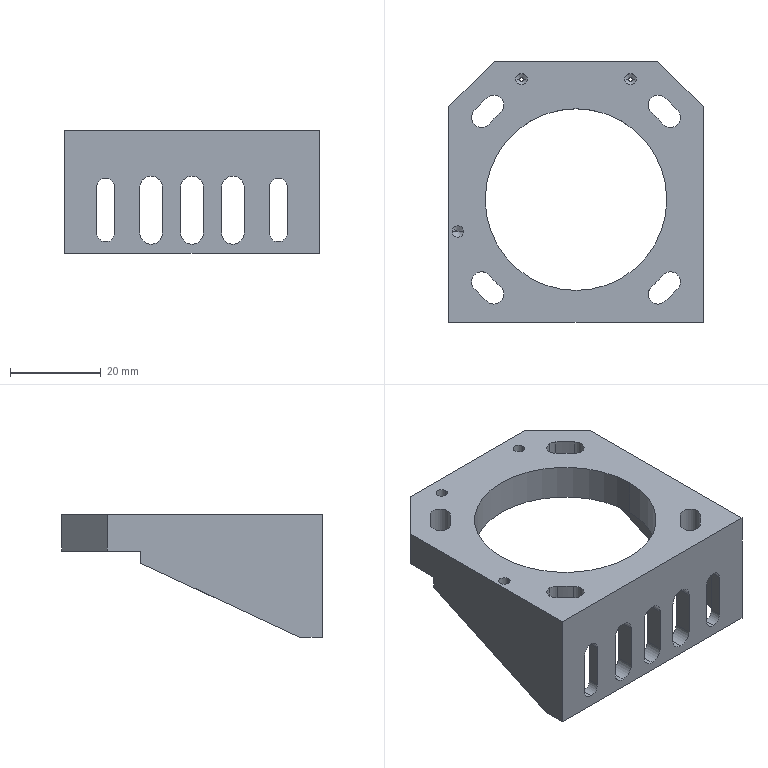NC program | NX | posted with a generic post | part box 56 x 57.4 x 27 mm
Lines 2971 to 3091 of 3091:
(PLANAR_MILL_COPY_COPY_COPY_1 , TOOL : D6A45)
N5934 T07 M6
N5936 G54
N5938 G17 G0 G90 X-1.555 Y-19.935 B0. C0. S7500 M3
N5940 G43 Z30. H7
N5942 Z0.5
N5944 G94 G1 X-1.259 Y-20.1 Z0.409 F1250.
N5946 X4. Z-1.
N5948 X9.
N5950 G3 X10.1 Y-19. R1.1
N5952 X9. Y-17.9 R1.1
N5954 G1 X-1.
N5956 G3 X-2.1 Y-19. R1.1
N5958 X-1. Y-20.1 R1.1
N5960 G1 X4.
N5962 G3 X4.866 Y-19.6 R1.
N5964 G1 Z0.5
N5966 G0 Z30.
N5968 X2.73 Y-9.4
N5970 Z0.5
N5972 G1 Z-1.
N5974 X3.134 Y-10.1
N5976 G3 X4. Y-10.6 R1.
N5978 G1 X9.
N5980 G3 X10.6 Y-9. R1.6
N5982 X9. Y-7.4 R1.6
N5984 G1 X-1.
N5986 G3 X-2.6 Y-9. R1.6
N5988 X-1. Y-10.6 R1.6
N5990 G1 X4.
N5992 G3 X4.866 Y-10.1 R1.
N5994 G1 X5.27 Y-9.4
N5996 Z0.5
N5998 G0 Z30.
N6000 X2.73 Y-0.4
N6002 Z0.5
N6004 G1 Z-1.
N6006 X3.134 Y-1.1
N6008 G3 X4. Y-1.6 R1.
N6010 G1 X9.
N6012 G3 X10.6 Y0. R1.6
N6014 X9. Y1.6 R1.6
N6016 G1 X-1.
N6018 G3 X-2.6 Y0. R1.6
N6020 X-1. Y-1.6 R1.6
N6022 G1 X4.
N6024 G3 X4.866 Y-1.1 R1.
N6026 G1 X5.27 Y-0.4
N6028 Z0.5
N6030 G0 Z30.
N6032 X2.73 Y8.6
N6034 Z0.5
N6036 G1 Z-1.
N6038 X3.134 Y7.9
N6040 G3 X4. Y7.4 R1.
N6042 G1 X9.
N6044 G3 X10.6 Y9. R1.6
N6046 X9. Y10.6 R1.6
N6048 G1 X-1.
N6050 G3 X-2.6 Y9. R1.6
N6052 X-1. Y7.4 R1.6
N6054 G1 X4.
N6056 G3 X4.866 Y7.9 R1.
N6058 G1 X5.27 Y8.6
N6060 Z0.5
N6062 G0 Z30.
N6064 X9.555 Y19.935
N6066 Z0.5
N6068 G1 X9.259 Y20.1 Z0.409
N6070 X4. Z-1.
N6072 X-1.
N6074 G3 X-2.1 Y19. R1.1
N6076 X-1. Y17.9 R1.1
N6078 G1 X9.
N6080 G3 X10.1 Y19. R1.1
N6082 X9. Y20.1 R1.1
N6084 G1 X4.
N6086 G3 X3.134 Y19.6 R1.
N6088 G1 Z0.5
N6090 G0 Z30.
N6092 M5
(刀补 , TOOL : D3)
N6094 T03 M6
N6096 G54
N6098 G17 G0 G90 X9.098 Y19.433 B0. C0. S7500 M3
N6100 G43 Z30. H3
N6102 Z1.
N6104 G94 G1 Z-4. F1000.
N6106 G41 X9. Y19.45 D3
N6108 X-1.
N6110 G3 X-1.45 Y19. R0.45
N6112 X-1. Y18.55 R0.45
N6114 G1 X9.
N6116 G3 X9.45 Y19. R0.45
N6118 X9. Y19.45 R0.45
N6120 X8.74 Y19.3 R0.3
N6122 G40
N6124 G1 X8.706 Y19.206
N6126 Z-3.
N6128 G0 Z30.
N6130 X-1.098 Y-19.433
N6132 Z1.
N6134 G1 Z-4.
N6136 G41 X-1. Y-19.45
N6138 X9.
N6140 G3 X9.45 Y-19. R0.45
N6142 X9. Y-18.55 R0.45
N6144 G1 X-1.
N6146 G3 X-1.45 Y-19. R0.45
N6148 X-1. Y-19.45 R0.45
N6150 X-0.74 Y-19.3 R0.3
N6152 G40
N6154 G1 X-0.706 Y-19.206
N6156 Z-3.
N6158 G0 Z30.
N6160 M5
N6162 M2